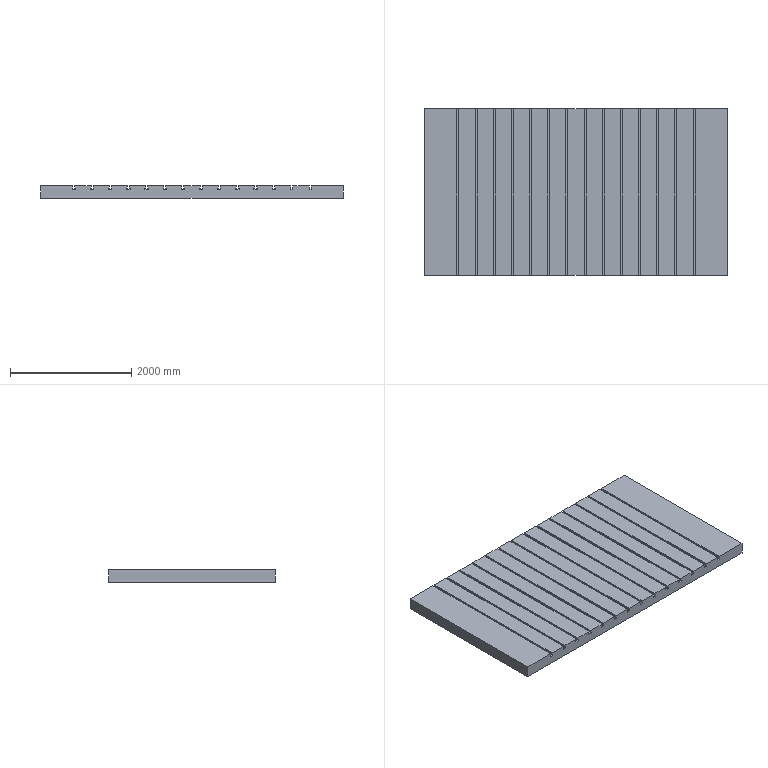Part | NX | features solid 2 | 1 solid | 110 faces | box 5000 x 2750 x 200 mm | volume 2665036000 mm3 | plane 110